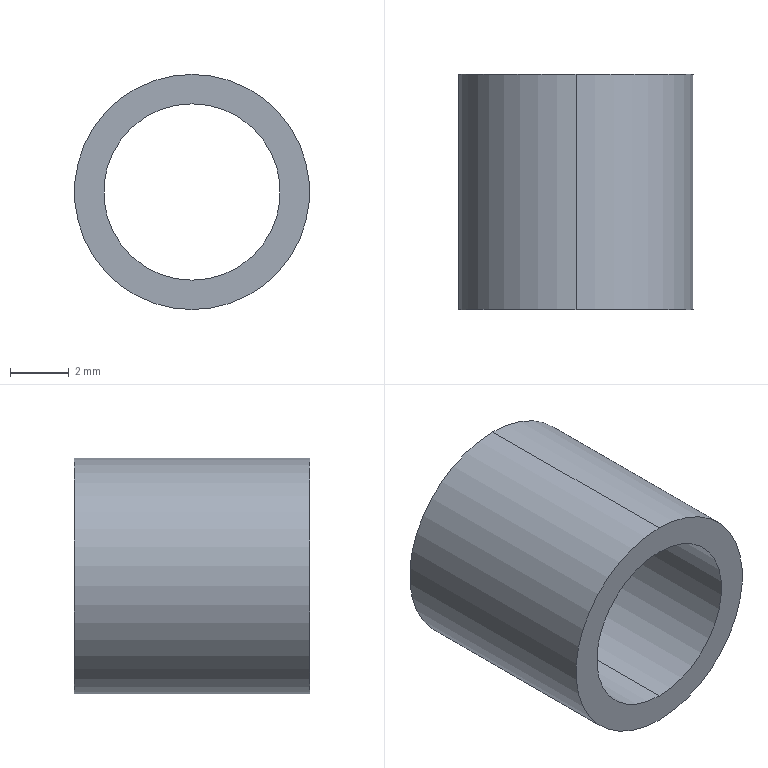Part | SolidWorks | features Extrusion 1 | 1 solid | 6 faces | box 8 x 8 x 8 mm | volume 175.929 mm3 | cylinder 4 | plane 2 | commonest cylinder face diameters 6 x2 8 x2
STEP:
#1=CARTESIAN_POINT('',(0.,8.,-3.));
#2=VERTEX_POINT('',#1);
#3=CARTESIAN_POINT('',(0.,8.,3.));
#4=VERTEX_POINT('',#3);
#5=CARTESIAN_POINT('',(0.,8.,0.));
#6=DIRECTION('',(0.,1.,0.));
#7=DIRECTION('',(0.,0.,1.));
#8=AXIS2_PLACEMENT_3D('',#5,#6,#7);
#9=CIRCLE('',#8,3.);
#10=EDGE_CURVE('',#2,#4,#9,.T.);
#11=ORIENTED_EDGE('',*,*,#10,.T.);
#12=CARTESIAN_POINT('',(0.,0.,3.));
#13=VERTEX_POINT('',#12);
#14=CARTESIAN_POINT('',(0.,8.,3.));
#15=DIRECTION('',(0.,-1.,0.));
#16=VECTOR('',#15,1000.);
#17=LINE('',#14,#16);
#18=EDGE_CURVE('',#4,#13,#17,.T.);
#19=ORIENTED_EDGE('',*,*,#18,.T.);
#20=CARTESIAN_POINT('',(0.,0.,-3.));
#21=VERTEX_POINT('',#20);
#22=CARTESIAN_POINT('',(0.,0.,0.));
#23=DIRECTION('',(0.,1.,0.));
#24=DIRECTION('',(0.,0.,1.));
#25=AXIS2_PLACEMENT_3D('',#22,#23,#24);
#26=CIRCLE('',#25,3.);
#27=EDGE_CURVE('',#21,#13,#26,.T.);
#28=ORIENTED_EDGE('',*,*,#27,.F.);
#29=CARTESIAN_POINT('',(0.,8.,-3.));
#30=DIRECTION('',(0.,-1.,0.));
#31=VECTOR('',#30,1000.);
#32=LINE('',#29,#31);
#33=EDGE_CURVE('',#2,#21,#32,.T.);
#34=ORIENTED_EDGE('',*,*,#33,.F.);
#35=EDGE_LOOP('',(#11,#19,#28,#34));
#36=FACE_OUTER_BOUND('',#35,.T.);
#37=CARTESIAN_POINT('',(0.,8.,0.));
#38=DIRECTION('',(0.,-1.,0.));
#39=DIRECTION('',(0.,0.,-1.));
#40=AXIS2_PLACEMENT_3D('',#37,#38,#39);
#41=CYLINDRICAL_SURFACE('',#40,3.);
#42=ADVANCED_FACE('',(#36),#41,.F.);
#43=CARTESIAN_POINT('',(0.,8.,4.));
#44=VERTEX_POINT('',#43);
#45=CARTESIAN_POINT('',(0.,8.,-4.));
#46=VERTEX_POINT('',#45);
#47=CARTESIAN_POINT('',(0.,8.,0.));
#48=DIRECTION('',(0.,1.,0.));
#49=DIRECTION('',(0.,0.,1.));
#50=AXIS2_PLACEMENT_3D('',#47,#48,#49);
#51=CIRCLE('',#50,4.);
#52=EDGE_CURVE('',#44,#46,#51,.T.);
#53=ORIENTED_EDGE('',*,*,#52,.F.);
#54=CARTESIAN_POINT('',(0.,0.,4.));
#55=VERTEX_POINT('',#54);
#56=CARTESIAN_POINT('',(0.,8.,4.));
#57=DIRECTION('',(0.,-1.,0.));
#58=VECTOR('',#57,1000.);
#59=LINE('',#56,#58);
#60=EDGE_CURVE('',#44,#55,#59,.T.);
#61=ORIENTED_EDGE('',*,*,#60,.T.);
#62=CARTESIAN_POINT('',(0.,0.,-4.));
#63=VERTEX_POINT('',#62);
#64=CARTESIAN_POINT('',(0.,0.,0.));
#65=DIRECTION('',(0.,1.,0.));
#66=DIRECTION('',(0.,0.,1.));
#67=AXIS2_PLACEMENT_3D('',#64,#65,#66);
#68=CIRCLE('',#67,4.);
#69=EDGE_CURVE('',#55,#63,#68,.T.);
#70=ORIENTED_EDGE('',*,*,#69,.T.);
#71=CARTESIAN_POINT('',(0.,8.,-4.));
#72=DIRECTION('',(0.,-1.,0.));
#73=VECTOR('',#72,1000.);
#74=LINE('',#71,#73);
#75=EDGE_CURVE('',#46,#63,#74,.T.);
#76=ORIENTED_EDGE('',*,*,#75,.F.);
#77=EDGE_LOOP('',(#53,#61,#70,#76));
#78=FACE_OUTER_BOUND('',#77,.T.);
#79=CARTESIAN_POINT('',(0.,8.,0.));
#80=DIRECTION('',(0.,-1.,0.));
#81=DIRECTION('',(0.,0.,-1.));
#82=AXIS2_PLACEMENT_3D('',#79,#80,#81);
#83=CYLINDRICAL_SURFACE('',#82,4.);
#84=ADVANCED_FACE('',(#78),#83,.T.);
#85=CARTESIAN_POINT('',(0.,8.,0.));
#86=DIRECTION('',(0.,1.,0.));
#87=DIRECTION('',(0.,0.,1.));
#88=AXIS2_PLACEMENT_3D('',#85,#86,#87);
#89=CIRCLE('',#88,4.);
#90=EDGE_CURVE('',#46,#44,#89,.T.);
#91=ORIENTED_EDGE('',*,*,#90,.T.);
#92=ORIENTED_EDGE('',*,*,#52,.T.);
#93=EDGE_LOOP('',(#91,#92));
#94=FACE_OUTER_BOUND('',#93,.T.);
#95=ORIENTED_EDGE('',*,*,#10,.F.);
#96=CARTESIAN_POINT('',(0.,8.,0.));
#97=DIRECTION('',(0.,1.,0.));
#98=DIRECTION('',(0.,0.,1.));
#99=AXIS2_PLACEMENT_3D('',#96,#97,#98);
#100=CIRCLE('',#99,3.);
#101=EDGE_CURVE('',#4,#2,#100,.T.);
#102=ORIENTED_EDGE('',*,*,#101,.F.);
#103=EDGE_LOOP('',(#95,#102));
#104=FACE_BOUND('',#103,.T.);
#105=CARTESIAN_POINT('',(0.,8.,0.));
#106=DIRECTION('',(0.,1.,0.));
#107=DIRECTION('',(0.,0.,1.));
#108=AXIS2_PLACEMENT_3D('',#105,#106,#107);
#109=PLANE('',#108);
#110=ADVANCED_FACE('',(#94,#104),#109,.T.);
#111=CARTESIAN_POINT('',(0.,0.,0.));
#112=DIRECTION('',(0.,1.,0.));
#113=DIRECTION('',(0.,0.,1.));
#114=AXIS2_PLACEMENT_3D('',#111,#112,#113);
#115=CIRCLE('',#114,4.);
#116=EDGE_CURVE('',#63,#55,#115,.T.);
#117=ORIENTED_EDGE('',*,*,#116,.F.);
#118=ORIENTED_EDGE('',*,*,#69,.F.);
#119=EDGE_LOOP('',(#117,#118));
#120=FACE_OUTER_BOUND('',#119,.T.);
#121=ORIENTED_EDGE('',*,*,#27,.T.);
#122=CARTESIAN_POINT('',(0.,0.,0.));
#123=DIRECTION('',(0.,1.,0.));
#124=DIRECTION('',(0.,0.,1.));
#125=AXIS2_PLACEMENT_3D('',#122,#123,#124);
#126=CIRCLE('',#125,3.);
#127=EDGE_CURVE('',#13,#21,#126,.T.);
#128=ORIENTED_EDGE('',*,*,#127,.T.);
#129=EDGE_LOOP('',(#121,#128));
#130=FACE_BOUND('',#129,.T.);
#131=CARTESIAN_POINT('',(0.,0.,0.));
#132=DIRECTION('',(0.,1.,0.));
#133=DIRECTION('',(0.,0.,1.));
#134=AXIS2_PLACEMENT_3D('',#131,#132,#133);
#135=PLANE('',#134);
#136=ADVANCED_FACE('',(#120,#130),#135,.F.);
#137=ORIENTED_EDGE('',*,*,#60,.F.);
#138=ORIENTED_EDGE('',*,*,#90,.F.);
#139=ORIENTED_EDGE('',*,*,#75,.T.);
#140=ORIENTED_EDGE('',*,*,#116,.T.);
#141=EDGE_LOOP('',(#137,#138,#139,#140));
#142=FACE_OUTER_BOUND('',#141,.T.);
#143=CARTESIAN_POINT('',(0.,8.,0.));
#144=DIRECTION('',(0.,-1.,0.));
#145=DIRECTION('',(0.,0.,-1.));
#146=AXIS2_PLACEMENT_3D('',#143,#144,#145);
#147=CYLINDRICAL_SURFACE('',#146,4.);
#148=ADVANCED_FACE('',(#142),#147,.T.);
#149=ORIENTED_EDGE('',*,*,#18,.F.);
#150=ORIENTED_EDGE('',*,*,#101,.T.);
#151=ORIENTED_EDGE('',*,*,#33,.T.);
#152=ORIENTED_EDGE('',*,*,#127,.F.);
#153=EDGE_LOOP('',(#149,#150,#151,#152));
#154=FACE_OUTER_BOUND('',#153,.T.);
#155=CARTESIAN_POINT('',(0.,8.,0.));
#156=DIRECTION('',(0.,-1.,0.));
#157=DIRECTION('',(0.,0.,-1.));
#158=AXIS2_PLACEMENT_3D('',#155,#156,#157);
#159=CYLINDRICAL_SURFACE('',#158,3.);
#160=ADVANCED_FACE('',(#154),#159,.F.);
#161=CLOSED_SHELL('',(#42,#84,#110,#136,#148,#160));
#162=MANIFOLD_SOLID_BREP('',#161);
#163=CARTESIAN_POINT('',(0.,0.,0.));
#164=DIRECTION('',(0.,0.,1.));
#165=DIRECTION('',(1.,0.,0.));
#166=AXIS2_PLACEMENT_3D('',#163,#164,#165);
#167=(LENGTH_UNIT()NAMED_UNIT(*)SI_UNIT(.MILLI.,.METRE.));
#168=UNCERTAINTY_MEASURE_WITH_UNIT(LENGTH_MEASURE(0.00001),#167,'','');
#169=(NAMED_UNIT(*)PLANE_ANGLE_UNIT()SI_UNIT($,.RADIAN.));
#170=(NAMED_UNIT(*)SI_UNIT($,.STERADIAN.)SOLID_ANGLE_UNIT());
#171=(GEOMETRIC_REPRESENTATION_CONTEXT(3)GLOBAL_UNCERTAINTY_ASSIGNED_CONTEXT((#168))GLOBAL_UNIT_ASSIGNED_CONTEXT((#167,#169,#170))REPRESENTATION_CONTEXT('',''));
#172=ADVANCED_BREP_SHAPE_REPRESENTATION('',(#162,#166),#171);